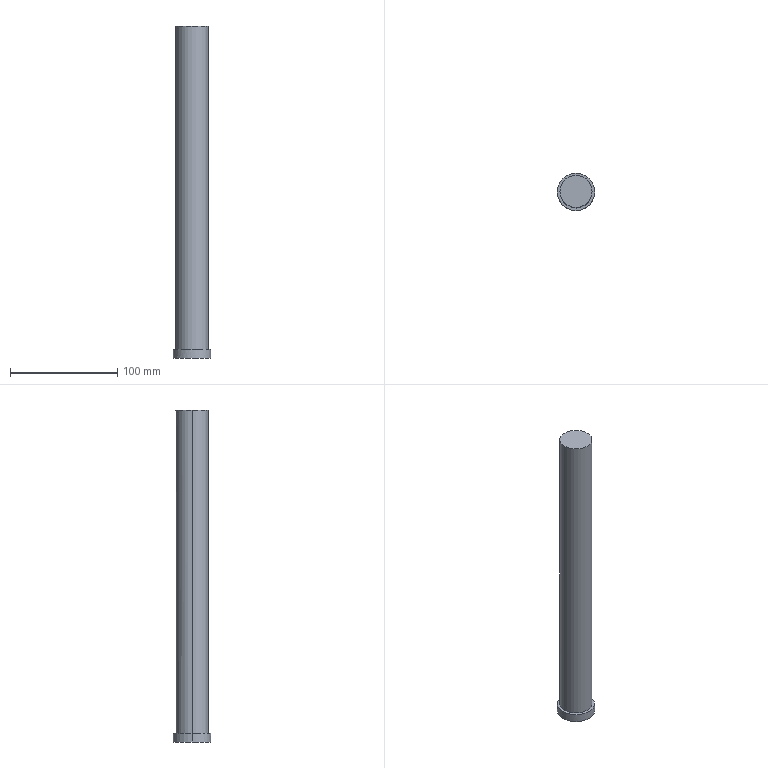Part | Creo | 1 solid | 7 faces | box 35 x 35 x 310 mm | volume 221168 mm3 | cylinder 4 | plane 3 | commonest cylinder face diameters 30 x2 35 x2
STEP:
#1=CARTESIAN_POINT('',(0.,0.,0.));
#2=DIRECTION('',(0.,0.,1.));
#3=DIRECTION('',(1.,0.,0.));
#4=AXIS2_PLACEMENT_3D('',#1,#2,#3);
#5=CARTESIAN_POINT('',(461.601,-277.627,-330.441));
#6=VERTEX_POINT('',#5);
#7=CARTESIAN_POINT('',(444.101,-260.127,-330.441));
#8=VERTEX_POINT('',#7);
#9=CARTESIAN_POINT('',(444.101,-277.627,-330.441));
#10=DIRECTION('',(0.,0.,1.));
#11=DIRECTION('',(1.,0.,0.));
#12=AXIS2_PLACEMENT_3D('',#9,#10,#11);
#13=CIRCLE('',#12,17.5);
#14=EDGE_CURVE('',#6,#8,#13,.T.);
#15=ORIENTED_EDGE('',*,*,#14,.T.);
#16=CARTESIAN_POINT('',(426.601,-277.627,-330.441));
#17=VERTEX_POINT('',#16);
#18=CARTESIAN_POINT('',(444.101,-277.627,-330.441));
#19=DIRECTION('',(0.,0.,1.));
#20=DIRECTION('',(0.,1.,0.));
#21=AXIS2_PLACEMENT_3D('',#18,#19,#20);
#22=CIRCLE('',#21,17.5);
#23=EDGE_CURVE('',#8,#17,#22,.T.);
#24=ORIENTED_EDGE('',*,*,#23,.T.);
#25=CARTESIAN_POINT('',(426.601,-277.627,-338.441));
#26=VERTEX_POINT('',#25);
#27=CARTESIAN_POINT('',(426.601,-277.627,-330.441));
#28=DIRECTION('',(0.,0.,-1.));
#29=VECTOR('',#28,8.);
#30=LINE('',#27,#29);
#31=EDGE_CURVE('',#17,#26,#30,.T.);
#32=ORIENTED_EDGE('',*,*,#31,.T.);
#33=CARTESIAN_POINT('',(444.101,-260.127,-338.441));
#34=VERTEX_POINT('',#33);
#35=CARTESIAN_POINT('',(444.101,-277.627,-338.441));
#36=DIRECTION('',(0.,0.,-1.));
#37=DIRECTION('',(-1.,0.,0.));
#38=AXIS2_PLACEMENT_3D('',#35,#36,#37);
#39=CIRCLE('',#38,17.5);
#40=EDGE_CURVE('',#26,#34,#39,.T.);
#41=ORIENTED_EDGE('',*,*,#40,.T.);
#42=CARTESIAN_POINT('',(461.601,-277.627,-338.441));
#43=VERTEX_POINT('',#42);
#44=CARTESIAN_POINT('',(444.101,-277.627,-338.441));
#45=DIRECTION('',(0.,0.,-1.));
#46=DIRECTION('',(0.,1.,0.));
#47=AXIS2_PLACEMENT_3D('',#44,#45,#46);
#48=CIRCLE('',#47,17.5);
#49=EDGE_CURVE('',#34,#43,#48,.T.);
#50=ORIENTED_EDGE('',*,*,#49,.T.);
#51=CARTESIAN_POINT('',(461.601,-277.627,-330.441));
#52=DIRECTION('',(0.,0.,-1.));
#53=VECTOR('',#52,8.);
#54=LINE('',#51,#53);
#55=EDGE_CURVE('',#6,#43,#54,.T.);
#56=ORIENTED_EDGE('',*,*,#55,.F.);
#57=EDGE_LOOP('',(#15,#24,#32,#41,#50,#56));
#58=FACE_OUTER_BOUND('',#57,.F.);
#59=CARTESIAN_POINT('',(444.101,-277.627,-330.441));
#60=DIRECTION('',(0.,0.,-1.));
#61=DIRECTION('',(-1.,0.,0.));
#62=AXIS2_PLACEMENT_3D('',#59,#60,#61);
#63=CYLINDRICAL_SURFACE('',#62,17.5);
#64=ADVANCED_FACE('',(#58),#63,.T.);
#65=ORIENTED_EDGE('',*,*,#23,.F.);
#66=ORIENTED_EDGE('',*,*,#14,.F.);
#67=CARTESIAN_POINT('',(444.101,-277.627,-330.441));
#68=DIRECTION('',(0.,0.,1.));
#69=DIRECTION('',(-1.,0.,0.));
#70=AXIS2_PLACEMENT_3D('',#67,#68,#69);
#71=CIRCLE('',#70,17.5);
#72=EDGE_CURVE('',#17,#6,#71,.T.);
#73=ORIENTED_EDGE('',*,*,#72,.F.);
#74=EDGE_LOOP('',(#65,#66,#73));
#75=FACE_OUTER_BOUND('',#74,.F.);
#76=CARTESIAN_POINT('',(444.101,-292.627,-330.441));
#77=VERTEX_POINT('',#76);
#78=CARTESIAN_POINT('',(429.101,-277.627,-330.441));
#79=VERTEX_POINT('',#78);
#80=CARTESIAN_POINT('',(444.101,-277.627,-330.441));
#81=DIRECTION('',(0.,0.,-1.));
#82=DIRECTION('',(0.,-1.,0.));
#83=AXIS2_PLACEMENT_3D('',#80,#81,#82);
#84=CIRCLE('',#83,15.);
#85=EDGE_CURVE('',#77,#79,#84,.T.);
#86=ORIENTED_EDGE('',*,*,#85,.F.);
#87=CARTESIAN_POINT('',(459.101,-277.627,-330.441));
#88=VERTEX_POINT('',#87);
#89=CARTESIAN_POINT('',(444.101,-277.627,-330.441));
#90=DIRECTION('',(0.,0.,-1.));
#91=DIRECTION('',(1.,0.,0.));
#92=AXIS2_PLACEMENT_3D('',#89,#90,#91);
#93=CIRCLE('',#92,15.);
#94=EDGE_CURVE('',#88,#77,#93,.T.);
#95=ORIENTED_EDGE('',*,*,#94,.F.);
#96=CARTESIAN_POINT('',(444.101,-277.627,-330.441));
#97=DIRECTION('',(0.,0.,-1.));
#98=DIRECTION('',(-1.,0.,0.));
#99=AXIS2_PLACEMENT_3D('',#96,#97,#98);
#100=CIRCLE('',#99,15.);
#101=EDGE_CURVE('',#79,#88,#100,.T.);
#102=ORIENTED_EDGE('',*,*,#101,.F.);
#103=EDGE_LOOP('',(#86,#95,#102));
#104=FACE_BOUND('',#103,.F.);
#105=CARTESIAN_POINT('',(444.101,-277.627,-330.441));
#106=DIRECTION('',(0.,0.,-1.));
#107=DIRECTION('',(-1.,0.,0.));
#108=AXIS2_PLACEMENT_3D('',#105,#106,#107);
#109=PLANE('',#108);
#110=ADVANCED_FACE('',(#75,#104),#109,.F.);
#111=CARTESIAN_POINT('',(429.101,-277.627,-28.441));
#112=VERTEX_POINT('',#111);
#113=CARTESIAN_POINT('',(444.101,-292.627,-28.441));
#114=VERTEX_POINT('',#113);
#115=CARTESIAN_POINT('',(444.101,-277.627,-28.441));
#116=DIRECTION('',(0.,0.,1.));
#117=DIRECTION('',(-1.,0.,0.));
#118=AXIS2_PLACEMENT_3D('',#115,#116,#117);
#119=CIRCLE('',#118,15.);
#120=EDGE_CURVE('',#112,#114,#119,.T.);
#121=ORIENTED_EDGE('',*,*,#120,.T.);
#122=CARTESIAN_POINT('',(459.101,-277.627,-28.441));
#123=VERTEX_POINT('',#122);
#124=CARTESIAN_POINT('',(444.101,-277.627,-28.441));
#125=DIRECTION('',(0.,0.,1.));
#126=DIRECTION('',(0.,-1.,0.));
#127=AXIS2_PLACEMENT_3D('',#124,#125,#126);
#128=CIRCLE('',#127,15.);
#129=EDGE_CURVE('',#114,#123,#128,.T.);
#130=ORIENTED_EDGE('',*,*,#129,.T.);
#131=CARTESIAN_POINT('',(459.101,-277.627,-330.441));
#132=DIRECTION('',(0.,0.,1.));
#133=VECTOR('',#132,302.);
#134=LINE('',#131,#133);
#135=EDGE_CURVE('',#88,#123,#134,.T.);
#136=ORIENTED_EDGE('',*,*,#135,.F.);
#137=ORIENTED_EDGE('',*,*,#94,.T.);
#138=ORIENTED_EDGE('',*,*,#85,.T.);
#139=CARTESIAN_POINT('',(429.101,-277.627,-330.441));
#140=DIRECTION('',(0.,0.,1.));
#141=VECTOR('',#140,302.);
#142=LINE('',#139,#141);
#143=EDGE_CURVE('',#79,#112,#142,.T.);
#144=ORIENTED_EDGE('',*,*,#143,.T.);
#145=EDGE_LOOP('',(#121,#130,#136,#137,#138,#144));
#146=FACE_OUTER_BOUND('',#145,.F.);
#147=CARTESIAN_POINT('',(444.101,-277.627,-330.441));
#148=DIRECTION('',(0.,0.,1.));
#149=DIRECTION('',(1.,0.,0.));
#150=AXIS2_PLACEMENT_3D('',#147,#148,#149);
#151=CYLINDRICAL_SURFACE('',#150,15.);
#152=ADVANCED_FACE('',(#146),#151,.T.);
#153=ORIENTED_EDGE('',*,*,#129,.F.);
#154=ORIENTED_EDGE('',*,*,#120,.F.);
#155=CARTESIAN_POINT('',(444.101,-262.627,-28.441));
#156=VERTEX_POINT('',#155);
#157=CARTESIAN_POINT('',(444.101,-277.627,-28.441));
#158=DIRECTION('',(0.,0.,1.));
#159=DIRECTION('',(0.,1.,0.));
#160=AXIS2_PLACEMENT_3D('',#157,#158,#159);
#161=CIRCLE('',#160,15.);
#162=EDGE_CURVE('',#156,#112,#161,.T.);
#163=ORIENTED_EDGE('',*,*,#162,.F.);
#164=CARTESIAN_POINT('',(444.101,-277.627,-28.441));
#165=DIRECTION('',(0.,0.,1.));
#166=DIRECTION('',(1.,0.,0.));
#167=AXIS2_PLACEMENT_3D('',#164,#165,#166);
#168=CIRCLE('',#167,15.);
#169=EDGE_CURVE('',#123,#156,#168,.T.);
#170=ORIENTED_EDGE('',*,*,#169,.F.);
#171=EDGE_LOOP('',(#153,#154,#163,#170));
#172=FACE_OUTER_BOUND('',#171,.F.);
#173=CARTESIAN_POINT('',(444.101,-277.627,-28.441));
#174=DIRECTION('',(0.,0.,1.));
#175=DIRECTION('',(1.,0.,0.));
#176=AXIS2_PLACEMENT_3D('',#173,#174,#175);
#177=PLANE('',#176);
#178=ADVANCED_FACE('',(#172),#177,.T.);
#179=ORIENTED_EDGE('',*,*,#162,.T.);
#180=ORIENTED_EDGE('',*,*,#143,.F.);
#181=ORIENTED_EDGE('',*,*,#101,.T.);
#182=ORIENTED_EDGE('',*,*,#135,.T.);
#183=ORIENTED_EDGE('',*,*,#169,.T.);
#184=EDGE_LOOP('',(#179,#180,#181,#182,#183));
#185=FACE_OUTER_BOUND('',#184,.F.);
#186=CARTESIAN_POINT('',(444.101,-277.627,-330.441));
#187=DIRECTION('',(0.,0.,1.));
#188=DIRECTION('',(1.,0.,0.));
#189=AXIS2_PLACEMENT_3D('',#186,#187,#188);
#190=CYLINDRICAL_SURFACE('',#189,15.);
#191=ADVANCED_FACE('',(#185),#190,.T.);
#192=ORIENTED_EDGE('',*,*,#72,.T.);
#193=ORIENTED_EDGE('',*,*,#55,.T.);
#194=CARTESIAN_POINT('',(444.101,-295.127,-338.441));
#195=VERTEX_POINT('',#194);
#196=CARTESIAN_POINT('',(444.101,-277.627,-338.441));
#197=DIRECTION('',(0.,0.,-1.));
#198=DIRECTION('',(1.,0.,0.));
#199=AXIS2_PLACEMENT_3D('',#196,#197,#198);
#200=CIRCLE('',#199,17.5);
#201=EDGE_CURVE('',#43,#195,#200,.T.);
#202=ORIENTED_EDGE('',*,*,#201,.T.);
#203=CARTESIAN_POINT('',(444.101,-277.627,-338.441));
#204=DIRECTION('',(0.,0.,-1.));
#205=DIRECTION('',(0.,-1.,0.));
#206=AXIS2_PLACEMENT_3D('',#203,#204,#205);
#207=CIRCLE('',#206,17.5);
#208=EDGE_CURVE('',#195,#26,#207,.T.);
#209=ORIENTED_EDGE('',*,*,#208,.T.);
#210=ORIENTED_EDGE('',*,*,#31,.F.);
#211=EDGE_LOOP('',(#192,#193,#202,#209,#210));
#212=FACE_OUTER_BOUND('',#211,.F.);
#213=CARTESIAN_POINT('',(444.101,-277.627,-330.441));
#214=DIRECTION('',(0.,0.,-1.));
#215=DIRECTION('',(-1.,0.,0.));
#216=AXIS2_PLACEMENT_3D('',#213,#214,#215);
#217=CYLINDRICAL_SURFACE('',#216,17.5);
#218=ADVANCED_FACE('',(#212),#217,.T.);
#219=ORIENTED_EDGE('',*,*,#49,.F.);
#220=ORIENTED_EDGE('',*,*,#40,.F.);
#221=ORIENTED_EDGE('',*,*,#208,.F.);
#222=ORIENTED_EDGE('',*,*,#201,.F.);
#223=EDGE_LOOP('',(#219,#220,#221,#222));
#224=FACE_OUTER_BOUND('',#223,.F.);
#225=CARTESIAN_POINT('',(444.101,-277.627,-338.441));
#226=DIRECTION('',(0.,0.,-1.));
#227=DIRECTION('',(-1.,0.,0.));
#228=AXIS2_PLACEMENT_3D('',#225,#226,#227);
#229=PLANE('',#228);
#230=ADVANCED_FACE('',(#224),#229,.T.);
#231=CLOSED_SHELL('',(#64,#110,#152,#178,#191,#218,#230));
#232=MANIFOLD_SOLID_BREP('',#231);
#233=(LENGTH_UNIT()NAMED_UNIT(*)SI_UNIT(.MILLI.,.METRE.));
#234=UNCERTAINTY_MEASURE_WITH_UNIT(LENGTH_MEASURE(0.03139),#233,'','');
#235=(NAMED_UNIT(*)PLANE_ANGLE_UNIT()SI_UNIT($,.RADIAN.));
#236=PLANE_ANGLE_MEASURE_WITH_UNIT(PLANE_ANGLE_MEASURE(0.01745),#235);
#237=(CONVERSION_BASED_UNIT('DEGREE',#236)NAMED_UNIT(*)PLANE_ANGLE_UNIT());
#238=(NAMED_UNIT(*)SI_UNIT($,.STERADIAN.)SOLID_ANGLE_UNIT());
#239=(GEOMETRIC_REPRESENTATION_CONTEXT(3)GLOBAL_UNCERTAINTY_ASSIGNED_CONTEXT((#234))GLOBAL_UNIT_ASSIGNED_CONTEXT((#233,#237,#238))REPRESENTATION_CONTEXT('',''));
#240=ADVANCED_BREP_SHAPE_REPRESENTATION('',(#4,#232),#239);